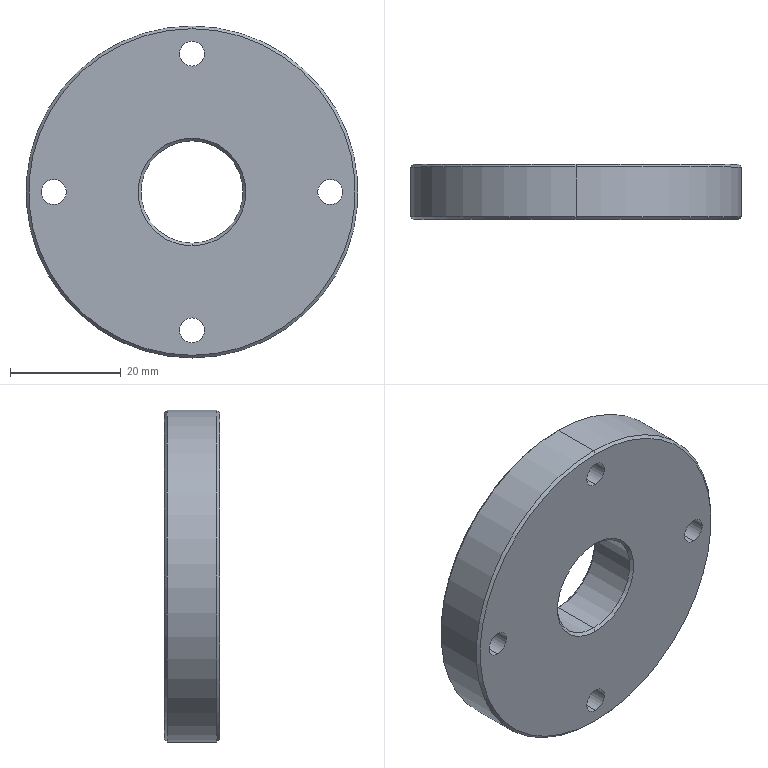Part | SolidWorks | features HoleWzd 2, Chamfer 1, Extrusion 1 | 1 solid | 34 faces | box 60 x 10 x 60 mm | volume 24256 mm3 | cylinder 20 | cone 8 | plane 6 | commonest cylinder face diameters 4.5 x8 8 x8 18.5 x2 60 x2
STEP:
#1=CARTESIAN_POINT('',(0.,10.,29.5));
#2=VERTEX_POINT('',#1);
#3=CARTESIAN_POINT('',(0.,10.,-29.5));
#4=VERTEX_POINT('',#3);
#5=CARTESIAN_POINT('',(0.,10.,0.));
#6=DIRECTION('',(0.,1.,0.));
#7=DIRECTION('',(0.,0.,1.));
#8=AXIS2_PLACEMENT_3D('',#5,#6,#7);
#9=CIRCLE('',#8,29.5);
#10=EDGE_CURVE('',#2,#4,#9,.T.);
#11=ORIENTED_EDGE('',*,*,#10,.F.);
#12=CARTESIAN_POINT('',(0.,9.5,30.));
#13=VERTEX_POINT('',#12);
#14=CARTESIAN_POINT('',(0.,10.,29.5));
#15=DIRECTION('',(0.,-0.7071,0.7071));
#16=VECTOR('',#15,1000.);
#17=LINE('',#14,#16);
#18=EDGE_CURVE('',#2,#13,#17,.T.);
#19=ORIENTED_EDGE('',*,*,#18,.T.);
#20=CARTESIAN_POINT('',(0.,9.5,-30.));
#21=VERTEX_POINT('',#20);
#22=CARTESIAN_POINT('',(0.,9.5,0.));
#23=DIRECTION('',(0.,-1.,0.));
#24=DIRECTION('',(0.,0.,1.));
#25=AXIS2_PLACEMENT_3D('',#22,#23,#24);
#26=CIRCLE('',#25,30.);
#27=EDGE_CURVE('',#21,#13,#26,.T.);
#28=ORIENTED_EDGE('',*,*,#27,.F.);
#29=CARTESIAN_POINT('',(0.,10.,-29.5));
#30=DIRECTION('',(0.,-0.7071,-0.7071));
#31=VECTOR('',#30,1000.);
#32=LINE('',#29,#31);
#33=EDGE_CURVE('',#4,#21,#32,.T.);
#34=ORIENTED_EDGE('',*,*,#33,.F.);
#35=EDGE_LOOP('',(#11,#19,#28,#34));
#36=FACE_OUTER_BOUND('',#35,.T.);
#37=CARTESIAN_POINT('',(0.,10.,0.));
#38=DIRECTION('',(0.,-1.,0.));
#39=DIRECTION('',(0.,0.,-1.));
#40=AXIS2_PLACEMENT_3D('',#37,#38,#39);
#41=CONICAL_SURFACE('',#40,29.5,0.7854);
#42=ADVANCED_FACE('',(#36),#41,.T.);
#43=CARTESIAN_POINT('',(0.,0.,-29.5));
#44=VERTEX_POINT('',#43);
#45=CARTESIAN_POINT('',(0.,0.,29.5));
#46=VERTEX_POINT('',#45);
#47=CARTESIAN_POINT('',(0.,0.,0.));
#48=DIRECTION('',(0.,-1.,0.));
#49=DIRECTION('',(0.,0.,1.));
#50=AXIS2_PLACEMENT_3D('',#47,#48,#49);
#51=CIRCLE('',#50,29.5);
#52=EDGE_CURVE('',#44,#46,#51,.T.);
#53=ORIENTED_EDGE('',*,*,#52,.F.);
#54=CARTESIAN_POINT('',(0.,0.5,-30.));
#55=VERTEX_POINT('',#54);
#56=CARTESIAN_POINT('',(0.,0.5,-30.));
#57=DIRECTION('',(0.,0.7071,-0.7071));
#58=VECTOR('',#57,1000.);
#59=LINE('',#56,#58);
#60=EDGE_CURVE('',#44,#55,#59,.T.);
#61=ORIENTED_EDGE('',*,*,#60,.T.);
#62=CARTESIAN_POINT('',(0.,0.5,30.));
#63=VERTEX_POINT('',#62);
#64=CARTESIAN_POINT('',(0.,0.5,0.));
#65=DIRECTION('',(0.,1.,0.));
#66=DIRECTION('',(0.,0.,1.));
#67=AXIS2_PLACEMENT_3D('',#64,#65,#66);
#68=CIRCLE('',#67,30.);
#69=EDGE_CURVE('',#63,#55,#68,.T.);
#70=ORIENTED_EDGE('',*,*,#69,.F.);
#71=CARTESIAN_POINT('',(0.,0.5,30.));
#72=DIRECTION('',(0.,0.7071,0.7071));
#73=VECTOR('',#72,1000.);
#74=LINE('',#71,#73);
#75=EDGE_CURVE('',#46,#63,#74,.T.);
#76=ORIENTED_EDGE('',*,*,#75,.F.);
#77=EDGE_LOOP('',(#53,#61,#70,#76));
#78=FACE_OUTER_BOUND('',#77,.T.);
#79=CARTESIAN_POINT('',(0.,0.5,0.));
#80=DIRECTION('',(0.,1.,0.));
#81=DIRECTION('',(0.,0.,1.));
#82=AXIS2_PLACEMENT_3D('',#79,#80,#81);
#83=CONICAL_SURFACE('',#82,30.,0.7854);
#84=ADVANCED_FACE('',(#78),#83,.T.);
#85=CARTESIAN_POINT('',(0.,9.5,-9.25));
#86=VERTEX_POINT('',#85);
#87=CARTESIAN_POINT('',(0.,9.5,9.25));
#88=VERTEX_POINT('',#87);
#89=CARTESIAN_POINT('',(0.,9.5,0.));
#90=DIRECTION('',(0.,1.,0.));
#91=DIRECTION('',(0.,0.,1.));
#92=AXIS2_PLACEMENT_3D('',#89,#90,#91);
#93=CIRCLE('',#92,9.25);
#94=EDGE_CURVE('',#86,#88,#93,.T.);
#95=ORIENTED_EDGE('',*,*,#94,.F.);
#96=CARTESIAN_POINT('',(0.,10.,-9.75));
#97=VERTEX_POINT('',#96);
#98=CARTESIAN_POINT('',(0.,9.5,-9.25));
#99=DIRECTION('',(0.,0.7071,-0.7071));
#100=VECTOR('',#99,1000.);
#101=LINE('',#98,#100);
#102=EDGE_CURVE('',#86,#97,#101,.T.);
#103=ORIENTED_EDGE('',*,*,#102,.T.);
#104=CARTESIAN_POINT('',(0.,10.,9.75));
#105=VERTEX_POINT('',#104);
#106=CARTESIAN_POINT('',(0.,10.,0.));
#107=DIRECTION('',(0.,-1.,0.));
#108=DIRECTION('',(0.,0.,1.));
#109=AXIS2_PLACEMENT_3D('',#106,#107,#108);
#110=CIRCLE('',#109,9.75);
#111=EDGE_CURVE('',#105,#97,#110,.T.);
#112=ORIENTED_EDGE('',*,*,#111,.F.);
#113=CARTESIAN_POINT('',(0.,9.5,9.25));
#114=DIRECTION('',(0.,0.7071,0.7071));
#115=VECTOR('',#114,1000.);
#116=LINE('',#113,#115);
#117=EDGE_CURVE('',#88,#105,#116,.T.);
#118=ORIENTED_EDGE('',*,*,#117,.F.);
#119=EDGE_LOOP('',(#95,#103,#112,#118));
#120=FACE_OUTER_BOUND('',#119,.T.);
#121=CARTESIAN_POINT('',(0.,9.5,0.));
#122=DIRECTION('',(0.,1.,0.));
#123=DIRECTION('',(0.,0.,1.));
#124=AXIS2_PLACEMENT_3D('',#121,#122,#123);
#125=CONICAL_SURFACE('',#124,9.25,0.7854);
#126=ADVANCED_FACE('',(#120),#125,.F.);
#127=CARTESIAN_POINT('',(0.,0.5,9.25));
#128=VERTEX_POINT('',#127);
#129=CARTESIAN_POINT('',(0.,0.5,-9.25));
#130=VERTEX_POINT('',#129);
#131=CARTESIAN_POINT('',(0.,0.5,0.));
#132=DIRECTION('',(0.,-1.,0.));
#133=DIRECTION('',(0.,0.,1.));
#134=AXIS2_PLACEMENT_3D('',#131,#132,#133);
#135=CIRCLE('',#134,9.25);
#136=EDGE_CURVE('',#128,#130,#135,.T.);
#137=ORIENTED_EDGE('',*,*,#136,.F.);
#138=CARTESIAN_POINT('',(0.,0.,9.75));
#139=VERTEX_POINT('',#138);
#140=CARTESIAN_POINT('',(0.,0.,9.75));
#141=DIRECTION('',(0.,-0.7071,0.7071));
#142=VECTOR('',#141,1000.);
#143=LINE('',#140,#142);
#144=EDGE_CURVE('',#128,#139,#143,.T.);
#145=ORIENTED_EDGE('',*,*,#144,.T.);
#146=CARTESIAN_POINT('',(0.,0.,-9.75));
#147=VERTEX_POINT('',#146);
#148=CARTESIAN_POINT('',(0.,0.,0.));
#149=DIRECTION('',(0.,1.,0.));
#150=DIRECTION('',(0.,0.,1.));
#151=AXIS2_PLACEMENT_3D('',#148,#149,#150);
#152=CIRCLE('',#151,9.75);
#153=EDGE_CURVE('',#147,#139,#152,.T.);
#154=ORIENTED_EDGE('',*,*,#153,.F.);
#155=CARTESIAN_POINT('',(0.,0.,-9.75));
#156=DIRECTION('',(0.,-0.7071,-0.7071));
#157=VECTOR('',#156,1000.);
#158=LINE('',#155,#157);
#159=EDGE_CURVE('',#130,#147,#158,.T.);
#160=ORIENTED_EDGE('',*,*,#159,.F.);
#161=EDGE_LOOP('',(#137,#145,#154,#160));
#162=FACE_OUTER_BOUND('',#161,.T.);
#163=CARTESIAN_POINT('',(0.,0.,0.));
#164=DIRECTION('',(0.,-1.,0.));
#165=DIRECTION('',(0.,0.,-1.));
#166=AXIS2_PLACEMENT_3D('',#163,#164,#165);
#167=CONICAL_SURFACE('',#166,9.75,0.7854);
#168=ADVANCED_FACE('',(#162),#167,.F.);
#169=CARTESIAN_POINT('',(0.,5.4,-29.));
#170=VERTEX_POINT('',#169);
#171=CARTESIAN_POINT('',(0.,5.4,-21.));
#172=VERTEX_POINT('',#171);
#173=CARTESIAN_POINT('',(0.,5.4,-25.));
#174=DIRECTION('',(0.,1.,0.));
#175=DIRECTION('',(0.,0.,1.));
#176=AXIS2_PLACEMENT_3D('',#173,#174,#175);
#177=CIRCLE('',#176,4.);
#178=EDGE_CURVE('',#170,#172,#177,.T.);
#179=ORIENTED_EDGE('',*,*,#178,.F.);
#180=CARTESIAN_POINT('',(0.,10.,-29.));
#181=VERTEX_POINT('',#180);
#182=CARTESIAN_POINT('',(0.,10.,-29.));
#183=DIRECTION('',(0.,1.,0.));
#184=VECTOR('',#183,1000.);
#185=LINE('',#182,#184);
#186=EDGE_CURVE('',#170,#181,#185,.T.);
#187=ORIENTED_EDGE('',*,*,#186,.T.);
#188=CARTESIAN_POINT('',(0.,10.,-21.));
#189=VERTEX_POINT('',#188);
#190=CARTESIAN_POINT('',(0.,10.,-25.));
#191=DIRECTION('',(0.,1.,0.));
#192=DIRECTION('',(0.,0.,1.));
#193=AXIS2_PLACEMENT_3D('',#190,#191,#192);
#194=CIRCLE('',#193,4.);
#195=EDGE_CURVE('',#181,#189,#194,.T.);
#196=ORIENTED_EDGE('',*,*,#195,.T.);
#197=CARTESIAN_POINT('',(0.,10.,-21.));
#198=DIRECTION('',(0.,1.,0.));
#199=VECTOR('',#198,1000.);
#200=LINE('',#197,#199);
#201=EDGE_CURVE('',#172,#189,#200,.T.);
#202=ORIENTED_EDGE('',*,*,#201,.F.);
#203=EDGE_LOOP('',(#179,#187,#196,#202));
#204=FACE_OUTER_BOUND('',#203,.T.);
#205=CARTESIAN_POINT('',(0.,10.,-25.));
#206=DIRECTION('',(0.,1.,0.));
#207=DIRECTION('',(0.,0.,1.));
#208=AXIS2_PLACEMENT_3D('',#205,#206,#207);
#209=CYLINDRICAL_SURFACE('',#208,4.);
#210=ADVANCED_FACE('',(#204),#209,.F.);
#211=CARTESIAN_POINT('',(0.,0.,-27.25));
#212=VERTEX_POINT('',#211);
#213=CARTESIAN_POINT('',(0.,0.,-22.75));
#214=VERTEX_POINT('',#213);
#215=CARTESIAN_POINT('',(0.,0.,-25.));
#216=DIRECTION('',(0.,1.,0.));
#217=DIRECTION('',(0.,0.,1.));
#218=AXIS2_PLACEMENT_3D('',#215,#216,#217);
#219=CIRCLE('',#218,2.25);
#220=EDGE_CURVE('',#212,#214,#219,.T.);
#221=ORIENTED_EDGE('',*,*,#220,.F.);
#222=CARTESIAN_POINT('',(0.,5.4,-27.25));
#223=VERTEX_POINT('',#222);
#224=CARTESIAN_POINT('',(0.,10.,-27.25));
#225=DIRECTION('',(0.,1.,0.));
#226=VECTOR('',#225,1000.);
#227=LINE('',#224,#226);
#228=EDGE_CURVE('',#212,#223,#227,.T.);
#229=ORIENTED_EDGE('',*,*,#228,.T.);
#230=CARTESIAN_POINT('',(0.,5.4,-22.75));
#231=VERTEX_POINT('',#230);
#232=CARTESIAN_POINT('',(0.,5.4,-25.));
#233=DIRECTION('',(0.,1.,0.));
#234=DIRECTION('',(0.,0.,1.));
#235=AXIS2_PLACEMENT_3D('',#232,#233,#234);
#236=CIRCLE('',#235,2.25);
#237=EDGE_CURVE('',#223,#231,#236,.T.);
#238=ORIENTED_EDGE('',*,*,#237,.T.);
#239=CARTESIAN_POINT('',(0.,10.,-22.75));
#240=DIRECTION('',(0.,1.,0.));
#241=VECTOR('',#240,1000.);
#242=LINE('',#239,#241);
#243=EDGE_CURVE('',#214,#231,#242,.T.);
#244=ORIENTED_EDGE('',*,*,#243,.F.);
#245=EDGE_LOOP('',(#221,#229,#238,#244));
#246=FACE_OUTER_BOUND('',#245,.T.);
#247=CARTESIAN_POINT('',(0.,10.,-25.));
#248=DIRECTION('',(0.,1.,0.));
#249=DIRECTION('',(0.,0.,1.));
#250=AXIS2_PLACEMENT_3D('',#247,#248,#249);
#251=CYLINDRICAL_SURFACE('',#250,2.25);
#252=ADVANCED_FACE('',(#246),#251,.F.);
#253=CARTESIAN_POINT('',(25.,5.4,-4.));
#254=VERTEX_POINT('',#253);
#255=CARTESIAN_POINT('',(25.,5.4,4.));
#256=VERTEX_POINT('',#255);
#257=CARTESIAN_POINT('',(25.,5.4,0.));
#258=DIRECTION('',(0.,1.,0.));
#259=DIRECTION('',(0.,0.,1.));
#260=AXIS2_PLACEMENT_3D('',#257,#258,#259);
#261=CIRCLE('',#260,4.);
#262=EDGE_CURVE('',#254,#256,#261,.T.);
#263=ORIENTED_EDGE('',*,*,#262,.F.);
#264=CARTESIAN_POINT('',(25.,10.,-4.));
#265=VERTEX_POINT('',#264);
#266=CARTESIAN_POINT('',(25.,10.,-4.));
#267=DIRECTION('',(0.,1.,0.));
#268=VECTOR('',#267,1000.);
#269=LINE('',#266,#268);
#270=EDGE_CURVE('',#254,#265,#269,.T.);
#271=ORIENTED_EDGE('',*,*,#270,.T.);
#272=CARTESIAN_POINT('',(25.,10.,4.));
#273=VERTEX_POINT('',#272);
#274=CARTESIAN_POINT('',(25.,10.,0.));
#275=DIRECTION('',(0.,1.,0.));
#276=DIRECTION('',(0.,0.,1.));
#277=AXIS2_PLACEMENT_3D('',#274,#275,#276);
#278=CIRCLE('',#277,4.);
#279=EDGE_CURVE('',#265,#273,#278,.T.);
#280=ORIENTED_EDGE('',*,*,#279,.T.);
#281=CARTESIAN_POINT('',(25.,10.,4.));
#282=DIRECTION('',(0.,1.,0.));
#283=VECTOR('',#282,1000.);
#284=LINE('',#281,#283);
#285=EDGE_CURVE('',#256,#273,#284,.T.);
#286=ORIENTED_EDGE('',*,*,#285,.F.);
#287=EDGE_LOOP('',(#263,#271,#280,#286));
#288=FACE_OUTER_BOUND('',#287,.T.);
#289=CARTESIAN_POINT('',(25.,10.,0.));
#290=DIRECTION('',(0.,1.,0.));
#291=DIRECTION('',(0.,0.,1.));
#292=AXIS2_PLACEMENT_3D('',#289,#290,#291);
#293=CYLINDRICAL_SURFACE('',#292,4.);
#294=ADVANCED_FACE('',(#288),#293,.F.);
#295=CARTESIAN_POINT('',(25.,0.,-2.25));
#296=VERTEX_POINT('',#295);
#297=CARTESIAN_POINT('',(25.,0.,2.25));
#298=VERTEX_POINT('',#297);
#299=CARTESIAN_POINT('',(25.,0.,0.));
#300=DIRECTION('',(0.,1.,0.));
#301=DIRECTION('',(0.,0.,1.));
#302=AXIS2_PLACEMENT_3D('',#299,#300,#301);
#303=CIRCLE('',#302,2.25);
#304=EDGE_CURVE('',#296,#298,#303,.T.);
#305=ORIENTED_EDGE('',*,*,#304,.F.);
#306=CARTESIAN_POINT('',(25.,5.4,-2.25));
#307=VERTEX_POINT('',#306);
#308=CARTESIAN_POINT('',(25.,10.,-2.25));
#309=DIRECTION('',(0.,1.,0.));
#310=VECTOR('',#309,1000.);
#311=LINE('',#308,#310);
#312=EDGE_CURVE('',#296,#307,#311,.T.);
#313=ORIENTED_EDGE('',*,*,#312,.T.);
#314=CARTESIAN_POINT('',(25.,5.4,2.25));
#315=VERTEX_POINT('',#314);
#316=CARTESIAN_POINT('',(25.,5.4,0.));
#317=DIRECTION('',(0.,1.,0.));
#318=DIRECTION('',(0.,0.,1.));
#319=AXIS2_PLACEMENT_3D('',#316,#317,#318);
#320=CIRCLE('',#319,2.25);
#321=EDGE_CURVE('',#307,#315,#320,.T.);
#322=ORIENTED_EDGE('',*,*,#321,.T.);
#323=CARTESIAN_POINT('',(25.,10.,2.25));
#324=DIRECTION('',(0.,1.,0.));
#325=VECTOR('',#324,1000.);
#326=LINE('',#323,#325);
#327=EDGE_CURVE('',#298,#315,#326,.T.);
#328=ORIENTED_EDGE('',*,*,#327,.F.);
#329=EDGE_LOOP('',(#305,#313,#322,#328));
#330=FACE_OUTER_BOUND('',#329,.T.);
#331=CARTESIAN_POINT('',(25.,10.,0.));
#332=DIRECTION('',(0.,1.,0.));
#333=DIRECTION('',(0.,0.,1.));
#334=AXIS2_PLACEMENT_3D('',#331,#332,#333);
#335=CYLINDRICAL_SURFACE('',#334,2.25);
#336=ADVANCED_FACE('',(#330),#335,.F.);
#337=CARTESIAN_POINT('',(0.,5.4,21.));
#338=VERTEX_POINT('',#337);
#339=CARTESIAN_POINT('',(0.,5.4,29.));
#340=VERTEX_POINT('',#339);
#341=CARTESIAN_POINT('',(0.,5.4,25.));
#342=DIRECTION('',(0.,1.,0.));
#343=DIRECTION('',(0.,0.,1.));
#344=AXIS2_PLACEMENT_3D('',#341,#342,#343);
#345=CIRCLE('',#344,4.);
#346=EDGE_CURVE('',#338,#340,#345,.T.);
#347=ORIENTED_EDGE('',*,*,#346,.F.);
#348=CARTESIAN_POINT('',(0.,10.,21.));
#349=VERTEX_POINT('',#348);
#350=CARTESIAN_POINT('',(0.,10.,21.));
#351=DIRECTION('',(0.,1.,0.));
#352=VECTOR('',#351,1000.);
#353=LINE('',#350,#352);
#354=EDGE_CURVE('',#338,#349,#353,.T.);
#355=ORIENTED_EDGE('',*,*,#354,.T.);
#356=CARTESIAN_POINT('',(0.,10.,29.));
#357=VERTEX_POINT('',#356);
#358=CARTESIAN_POINT('',(0.,10.,25.));
#359=DIRECTION('',(0.,1.,0.));
#360=DIRECTION('',(0.,0.,1.));
#361=AXIS2_PLACEMENT_3D('',#358,#359,#360);
#362=CIRCLE('',#361,4.);
#363=EDGE_CURVE('',#349,#357,#362,.T.);
#364=ORIENTED_EDGE('',*,*,#363,.T.);
#365=CARTESIAN_POINT('',(0.,10.,29.));
#366=DIRECTION('',(0.,1.,0.));
#367=VECTOR('',#366,1000.);
#368=LINE('',#365,#367);
#369=EDGE_CURVE('',#340,#357,#368,.T.);
#370=ORIENTED_EDGE('',*,*,#369,.F.);
#371=EDGE_LOOP('',(#347,#355,#364,#370));
#372=FACE_OUTER_BOUND('',#371,.T.);
#373=CARTESIAN_POINT('',(0.,10.,25.));
#374=DIRECTION('',(0.,1.,0.));
#375=DIRECTION('',(0.,0.,1.));
#376=AXIS2_PLACEMENT_3D('',#373,#374,#375);
#377=CYLINDRICAL_SURFACE('',#376,4.);
#378=ADVANCED_FACE('',(#372),#377,.F.);
#379=CARTESIAN_POINT('',(0.,0.,22.75));
#380=VERTEX_POINT('',#379);
#381=CARTESIAN_POINT('',(0.,0.,27.25));
#382=VERTEX_POINT('',#381);
#383=CARTESIAN_POINT('',(0.,0.,25.));
#384=DIRECTION('',(0.,1.,0.));
#385=DIRECTION('',(0.,0.,1.));
#386=AXIS2_PLACEMENT_3D('',#383,#384,#385);
#387=CIRCLE('',#386,2.25);
#388=EDGE_CURVE('',#380,#382,#387,.T.);
#389=ORIENTED_EDGE('',*,*,#388,.F.);
#390=CARTESIAN_POINT('',(0.,5.4,22.75));
#391=VERTEX_POINT('',#390);
#392=CARTESIAN_POINT('',(0.,10.,22.75));
#393=DIRECTION('',(0.,1.,0.));
#394=VECTOR('',#393,1000.);
#395=LINE('',#392,#394);
#396=EDGE_CURVE('',#380,#391,#395,.T.);
#397=ORIENTED_EDGE('',*,*,#396,.T.);
#398=CARTESIAN_POINT('',(0.,5.4,27.25));
#399=VERTEX_POINT('',#398);
#400=CARTESIAN_POINT('',(0.,5.4,25.));
#401=DIRECTION('',(0.,1.,0.));
#402=DIRECTION('',(0.,0.,1.));
#403=AXIS2_PLACEMENT_3D('',#400,#401,#402);
#404=CIRCLE('',#403,2.25);
#405=EDGE_CURVE('',#391,#399,#404,.T.);
#406=ORIENTED_EDGE('',*,*,#405,.T.);
#407=CARTESIAN_POINT('',(0.,10.,27.25));
#408=DIRECTION('',(0.,1.,0.));
#409=VECTOR('',#408,1000.);
#410=LINE('',#407,#409);
#411=EDGE_CURVE('',#382,#399,#410,.T.);
#412=ORIENTED_EDGE('',*,*,#411,.F.);
#413=EDGE_LOOP('',(#389,#397,#406,#412));
#414=FACE_OUTER_BOUND('',#413,.T.);
#415=CARTESIAN_POINT('',(0.,10.,25.));
#416=DIRECTION('',(0.,1.,0.));
#417=DIRECTION('',(0.,0.,1.));
#418=AXIS2_PLACEMENT_3D('',#415,#416,#417);
#419=CYLINDRICAL_SURFACE('',#418,2.25);
#420=ADVANCED_FACE('',(#414),#419,.F.);
#421=CARTESIAN_POINT('',(-25.,5.4,-4.));
#422=VERTEX_POINT('',#421);
#423=CARTESIAN_POINT('',(-25.,5.4,4.));
#424=VERTEX_POINT('',#423);
#425=CARTESIAN_POINT('',(-25.,5.4,0.));
#426=DIRECTION('',(0.,1.,0.));
#427=DIRECTION('',(0.,0.,1.));
#428=AXIS2_PLACEMENT_3D('',#425,#426,#427);
#429=CIRCLE('',#428,4.);
#430=EDGE_CURVE('',#422,#424,#429,.T.);
#431=ORIENTED_EDGE('',*,*,#430,.F.);
#432=CARTESIAN_POINT('',(-25.,10.,-4.));
#433=VERTEX_POINT('',#432);
#434=CARTESIAN_POINT('',(-25.,10.,-4.));
#435=DIRECTION('',(0.,1.,0.));
#436=VECTOR('',#435,1000.);
#437=LINE('',#434,#436);
#438=EDGE_CURVE('',#422,#433,#437,.T.);
#439=ORIENTED_EDGE('',*,*,#438,.T.);
#440=CARTESIAN_POINT('',(-25.,10.,4.));
#441=VERTEX_POINT('',#440);
#442=CARTESIAN_POINT('',(-25.,10.,0.));
#443=DIRECTION('',(0.,1.,0.));
#444=DIRECTION('',(0.,0.,1.));
#445=AXIS2_PLACEMENT_3D('',#442,#443,#444);
#446=CIRCLE('',#445,4.);
#447=EDGE_CURVE('',#433,#441,#446,.T.);
#448=ORIENTED_EDGE('',*,*,#447,.T.);
#449=CARTESIAN_POINT('',(-25.,10.,4.));
#450=DIRECTION('',(0.,1.,0.));
#451=VECTOR('',#450,1000.);
#452=LINE('',#449,#451);
#453=EDGE_CURVE('',#424,#441,#452,.T.);
#454=ORIENTED_EDGE('',*,*,#453,.F.);
#455=EDGE_LOOP('',(#431,#439,#448,#454));
#456=FACE_OUTER_BOUND('',#455,.T.);
#457=CARTESIAN_POINT('',(-25.,10.,0.));
#458=DIRECTION('',(0.,1.,0.));
#459=DIRECTION('',(0.,0.,1.));
#460=AXIS2_PLACEMENT_3D('',#457,#458,#459);
#461=CYLINDRICAL_SURFACE('',#460,4.);
#462=ADVANCED_FACE('',(#456),#461,.F.);
#463=CARTESIAN_POINT('',(-25.,0.,-2.25));
#464=VERTEX_POINT('',#463);
#465=CARTESIAN_POINT('',(-25.,0.,2.25));
#466=VERTEX_POINT('',#465);
#467=CARTESIAN_POINT('',(-25.,0.,0.));
#468=DIRECTION('',(0.,1.,0.));
#469=DIRECTION('',(0.,0.,1.));
#470=AXIS2_PLACEMENT_3D('',#467,#468,#469);
#471=CIRCLE('',#470,2.25);
#472=EDGE_CURVE('',#464,#466,#471,.T.);
#473=ORIENTED_EDGE('',*,*,#472,.F.);
#474=CARTESIAN_POINT('',(-25.,5.4,-2.25));
#475=VERTEX_POINT('',#474);
#476=CARTESIAN_POINT('',(-25.,10.,-2.25));
#477=DIRECTION('',(0.,1.,0.));
#478=VECTOR('',#477,1000.);
#479=LINE('',#476,#478);
#480=EDGE_CURVE('',#464,#475,#479,.T.);
#481=ORIENTED_EDGE('',*,*,#480,.T.);
#482=CARTESIAN_POINT('',(-25.,5.4,2.25));
#483=VERTEX_POINT('',#482);
#484=CARTESIAN_POINT('',(-25.,5.4,0.));
#485=DIRECTION('',(0.,1.,0.));
#486=DIRECTION('',(0.,0.,1.));
#487=AXIS2_PLACEMENT_3D('',#484,#485,#486);
#488=CIRCLE('',#487,2.25);
#489=EDGE_CURVE('',#475,#483,#488,.T.);
#490=ORIENTED_EDGE('',*,*,#489,.T.);
#491=CARTESIAN_POINT('',(-25.,10.,2.25));
#492=DIRECTION('',(0.,1.,0.));
#493=VECTOR('',#492,1000.);
#494=LINE('',#491,#493);
#495=EDGE_CURVE('',#466,#483,#494,.T.);
#496=ORIENTED_EDGE('',*,*,#495,.F.);
#497=EDGE_LOOP('',(#473,#481,#490,#496));
#498=FACE_OUTER_BOUND('',#497,.T.);
#499=CARTESIAN_POINT('',(-25.,10.,0.));
#500=DIRECTION('',(0.,1.,0.));
#501=DIRECTION('',(0.,0.,1.));
#502=AXIS2_PLACEMENT_3D('',#499,#500,#501);
#503=CYLINDRICAL_SURFACE('',#502,2.25);
#504=ADVANCED_FACE('',(#498),#503,.F.);
#505=ORIENTED_EDGE('',*,*,#136,.T.);
#506=CARTESIAN_POINT('',(0.,10.,-9.25));
#507=DIRECTION('',(0.,1.,0.));
#508=VECTOR('',#507,1000.);
#509=LINE('',#506,#508);
#510=EDGE_CURVE('',#130,#86,#509,.T.);
#511=ORIENTED_EDGE('',*,*,#510,.T.);
#512=ORIENTED_EDGE('',*,*,#94,.T.);
#513=CARTESIAN_POINT('',(0.,10.,9.25));
#514=DIRECTION('',(0.,1.,0.));
#515=VECTOR('',#514,1000.);
#516=LINE('',#513,#515);
#517=EDGE_CURVE('',#128,#88,#516,.T.);
#518=ORIENTED_EDGE('',*,*,#517,.F.);
#519=EDGE_LOOP('',(#505,#511,#512,#518));
#520=FACE_OUTER_BOUND('',#519,.T.);
#521=CARTESIAN_POINT('',(0.,10.,0.));
#522=DIRECTION('',(0.,1.,0.));
#523=DIRECTION('',(0.,0.,1.));
#524=AXIS2_PLACEMENT_3D('',#521,#522,#523);
#525=CYLINDRICAL_SURFACE('',#524,9.25);
#526=ADVANCED_FACE('',(#520),#525,.F.);
#527=ORIENTED_EDGE('',*,*,#27,.T.);
#528=CARTESIAN_POINT('',(0.,10.,30.));
#529=DIRECTION('',(0.,-1.,0.));
#530=VECTOR('',#529,1000.);
#531=LINE('',#528,#530);
#532=EDGE_CURVE('',#13,#63,#531,.T.);
#533=ORIENTED_EDGE('',*,*,#532,.T.);
#534=ORIENTED_EDGE('',*,*,#69,.T.);
#535=CARTESIAN_POINT('',(0.,10.,-30.));
#536=DIRECTION('',(0.,-1.,0.));
#537=VECTOR('',#536,1000.);
#538=LINE('',#535,#537);
#539=EDGE_CURVE('',#21,#55,#538,.T.);
#540=ORIENTED_EDGE('',*,*,#539,.F.);
#541=EDGE_LOOP('',(#527,#533,#534,#540));
#542=FACE_OUTER_BOUND('',#541,.T.);
#543=CARTESIAN_POINT('',(0.,10.,0.));
#544=DIRECTION('',(0.,-1.,0.));
#545=DIRECTION('',(0.,0.,-1.));
#546=AXIS2_PLACEMENT_3D('',#543,#544,#545);
#547=CYLINDRICAL_SURFACE('',#546,30.);
#548=ADVANCED_FACE('',(#542),#547,.T.);
#549=ORIENTED_EDGE('',*,*,#532,.F.);
#550=CARTESIAN_POINT('',(0.,9.5,0.));
#551=DIRECTION('',(0.,-1.,0.));
#552=DIRECTION('',(0.,0.,1.));
#553=AXIS2_PLACEMENT_3D('',#550,#551,#552);
#554=CIRCLE('',#553,30.);
#555=EDGE_CURVE('',#13,#21,#554,.T.);
#556=ORIENTED_EDGE('',*,*,#555,.T.);
#557=ORIENTED_EDGE('',*,*,#539,.T.);
#558=CARTESIAN_POINT('',(0.,0.5,0.));
#559=DIRECTION('',(0.,1.,0.));
#560=DIRECTION('',(0.,0.,1.));
#561=AXIS2_PLACEMENT_3D('',#558,#559,#560);
#562=CIRCLE('',#561,30.);
#563=EDGE_CURVE('',#55,#63,#562,.T.);
#564=ORIENTED_EDGE('',*,*,#563,.T.);
#565=EDGE_LOOP('',(#549,#556,#557,#564));
#566=FACE_OUTER_BOUND('',#565,.T.);
#567=CARTESIAN_POINT('',(0.,10.,0.));
#568=DIRECTION('',(0.,-1.,0.));
#569=DIRECTION('',(0.,0.,-1.));
#570=AXIS2_PLACEMENT_3D('',#567,#568,#569);
#571=CYLINDRICAL_SURFACE('',#570,30.);
#572=ADVANCED_FACE('',(#566),#571,.T.);
#573=ORIENTED_EDGE('',*,*,#111,.T.);
#574=CARTESIAN_POINT('',(0.,10.,0.));
#575=DIRECTION('',(0.,-1.,0.));
#576=DIRECTION('',(0.,0.,1.));
#577=AXIS2_PLACEMENT_3D('',#574,#575,#576);
#578=CIRCLE('',#577,9.75);
#579=EDGE_CURVE('',#97,#105,#578,.T.);
#580=ORIENTED_EDGE('',*,*,#579,.T.);
#581=EDGE_LOOP('',(#573,#580));
#582=FACE_BOUND('',#581,.T.);
#583=CARTESIAN_POINT('',(0.,10.,0.));
#584=DIRECTION('',(0.,1.,0.));
#585=DIRECTION('',(0.,0.,1.));
#586=AXIS2_PLACEMENT_3D('',#583,#584,#585);
#587=CIRCLE('',#586,29.5);
#588=EDGE_CURVE('',#4,#2,#587,.T.);
#589=ORIENTED_EDGE('',*,*,#588,.T.);
#590=ORIENTED_EDGE('',*,*,#10,.T.);
#591=EDGE_LOOP('',(#589,#590));
#592=FACE_OUTER_BOUND('',#591,.T.);
#593=CARTESIAN_POINT('',(0.,10.,-25.));
#594=DIRECTION('',(0.,1.,0.));
#595=DIRECTION('',(0.,0.,1.));
#596=AXIS2_PLACEMENT_3D('',#593,#594,#595);
#597=CIRCLE('',#596,4.);
#598=EDGE_CURVE('',#189,#181,#597,.T.);
#599=ORIENTED_EDGE('',*,*,#598,.F.);
#600=ORIENTED_EDGE('',*,*,#195,.F.);
#601=EDGE_LOOP('',(#599,#600));
#602=FACE_BOUND('',#601,.T.);
#603=CARTESIAN_POINT('',(25.,10.,0.));
#604=DIRECTION('',(0.,1.,0.));
#605=DIRECTION('',(0.,0.,1.));
#606=AXIS2_PLACEMENT_3D('',#603,#604,#605);
#607=CIRCLE('',#606,4.);
#608=EDGE_CURVE('',#273,#265,#607,.T.);
#609=ORIENTED_EDGE('',*,*,#608,.F.);
#610=ORIENTED_EDGE('',*,*,#279,.F.);
#611=EDGE_LOOP('',(#609,#610));
#612=FACE_BOUND('',#611,.T.);
#613=CARTESIAN_POINT('',(0.,10.,25.));
#614=DIRECTION('',(0.,1.,0.));
#615=DIRECTION('',(0.,0.,1.));
#616=AXIS2_PLACEMENT_3D('',#613,#614,#615);
#617=CIRCLE('',#616,4.);
#618=EDGE_CURVE('',#357,#349,#617,.T.);
#619=ORIENTED_EDGE('',*,*,#618,.F.);
#620=ORIENTED_EDGE('',*,*,#363,.F.);
#621=EDGE_LOOP('',(#619,#620));
#622=FACE_BOUND('',#621,.T.);
#623=CARTESIAN_POINT('',(-25.,10.,0.));
#624=DIRECTION('',(0.,1.,0.));
#625=DIRECTION('',(0.,0.,1.));
#626=AXIS2_PLACEMENT_3D('',#623,#624,#625);
#627=CIRCLE('',#626,4.);
#628=EDGE_CURVE('',#441,#433,#627,.T.);
#629=ORIENTED_EDGE('',*,*,#628,.F.);
#630=ORIENTED_EDGE('',*,*,#447,.F.);
#631=EDGE_LOOP('',(#629,#630));
#632=FACE_BOUND('',#631,.T.);
#633=CARTESIAN_POINT('',(0.,10.,0.));
#634=DIRECTION('',(0.,1.,0.));
#635=DIRECTION('',(0.,0.,1.));
#636=AXIS2_PLACEMENT_3D('',#633,#634,#635);
#637=PLANE('',#636);
#638=ADVANCED_FACE('',(#582,#592,#602,#612,#622,#632),#637,.T.);
#639=ORIENTED_EDGE('',*,*,#153,.T.);
#640=CARTESIAN_POINT('',(0.,0.,0.));
#641=DIRECTION('',(0.,1.,0.));
#642=DIRECTION('',(0.,0.,1.));
#643=AXIS2_PLACEMENT_3D('',#640,#641,#642);
#644=CIRCLE('',#643,9.75);
#645=EDGE_CURVE('',#139,#147,#644,.T.);
#646=ORIENTED_EDGE('',*,*,#645,.T.);
#647=EDGE_LOOP('',(#639,#646));
#648=FACE_BOUND('',#647,.T.);
#649=CARTESIAN_POINT('',(0.,0.,0.));
#650=DIRECTION('',(0.,-1.,0.));
#651=DIRECTION('',(0.,0.,1.));
#652=AXIS2_PLACEMENT_3D('',#649,#650,#651);
#653=CIRCLE('',#652,29.5);
#654=EDGE_CURVE('',#46,#44,#653,.T.);
#655=ORIENTED_EDGE('',*,*,#654,.T.);
#656=ORIENTED_EDGE('',*,*,#52,.T.);
#657=EDGE_LOOP('',(#655,#656));
#658=FACE_OUTER_BOUND('',#657,.T.);
#659=CARTESIAN_POINT('',(0.,0.,-25.));
#660=DIRECTION('',(0.,1.,0.));
#661=DIRECTION('',(0.,0.,1.));
#662=AXIS2_PLACEMENT_3D('',#659,#660,#661);
#663=CIRCLE('',#662,2.25);
#664=EDGE_CURVE('',#214,#212,#663,.T.);
#665=ORIENTED_EDGE('',*,*,#664,.T.);
#666=ORIENTED_EDGE('',*,*,#220,.T.);
#667=EDGE_LOOP('',(#665,#666));
#668=FACE_BOUND('',#667,.T.);
#669=CARTESIAN_POINT('',(25.,0.,0.));
#670=DIRECTION('',(0.,1.,0.));
#671=DIRECTION('',(0.,0.,1.));
#672=AXIS2_PLACEMENT_3D('',#669,#670,#671);
#673=CIRCLE('',#672,2.25);
#674=EDGE_CURVE('',#298,#296,#673,.T.);
#675=ORIENTED_EDGE('',*,*,#674,.T.);
#676=ORIENTED_EDGE('',*,*,#304,.T.);
#677=EDGE_LOOP('',(#675,#676));
#678=FACE_BOUND('',#677,.T.);
#679=CARTESIAN_POINT('',(0.,0.,25.));
#680=DIRECTION('',(0.,1.,0.));
#681=DIRECTION('',(0.,0.,1.));
#682=AXIS2_PLACEMENT_3D('',#679,#680,#681);
#683=CIRCLE('',#682,2.25);
#684=EDGE_CURVE('',#382,#380,#683,.T.);
#685=ORIENTED_EDGE('',*,*,#684,.T.);
#686=ORIENTED_EDGE('',*,*,#388,.T.);
#687=EDGE_LOOP('',(#685,#686));
#688=FACE_BOUND('',#687,.T.);
#689=CARTESIAN_POINT('',(-25.,0.,0.));
#690=DIRECTION('',(0.,1.,0.));
#691=DIRECTION('',(0.,0.,1.));
#692=AXIS2_PLACEMENT_3D('',#689,#690,#691);
#693=CIRCLE('',#692,2.25);
#694=EDGE_CURVE('',#466,#464,#693,.T.);
#695=ORIENTED_EDGE('',*,*,#694,.T.);
#696=ORIENTED_EDGE('',*,*,#472,.T.);
#697=EDGE_LOOP('',(#695,#696));
#698=FACE_BOUND('',#697,.T.);
#699=CARTESIAN_POINT('',(0.,0.,0.));
#700=DIRECTION('',(0.,1.,0.));
#701=DIRECTION('',(0.,0.,1.));
#702=AXIS2_PLACEMENT_3D('',#699,#700,#701);
#703=PLANE('',#702);
#704=ADVANCED_FACE('',(#648,#658,#668,#678,#688,#698),#703,.F.);
#705=ORIENTED_EDGE('',*,*,#510,.F.);
#706=CARTESIAN_POINT('',(0.,0.5,0.));
#707=DIRECTION('',(0.,-1.,0.));
#708=DIRECTION('',(0.,0.,1.));
#709=AXIS2_PLACEMENT_3D('',#706,#707,#708);
#710=CIRCLE('',#709,9.25);
#711=EDGE_CURVE('',#130,#128,#710,.T.);
#712=ORIENTED_EDGE('',*,*,#711,.T.);
#713=ORIENTED_EDGE('',*,*,#517,.T.);
#714=CARTESIAN_POINT('',(0.,9.5,0.));
#715=DIRECTION('',(0.,1.,0.));
#716=DIRECTION('',(0.,0.,1.));
#717=AXIS2_PLACEMENT_3D('',#714,#715,#716);
#718=CIRCLE('',#717,9.25);
#719=EDGE_CURVE('',#88,#86,#718,.T.);
#720=ORIENTED_EDGE('',*,*,#719,.T.);
#721=EDGE_LOOP('',(#705,#712,#713,#720));
#722=FACE_OUTER_BOUND('',#721,.T.);
#723=CARTESIAN_POINT('',(0.,10.,0.));
#724=DIRECTION('',(0.,1.,0.));
#725=DIRECTION('',(0.,0.,1.));
#726=AXIS2_PLACEMENT_3D('',#723,#724,#725);
#727=CYLINDRICAL_SURFACE('',#726,9.25);
#728=ADVANCED_FACE('',(#722),#727,.F.);
#729=ORIENTED_EDGE('',*,*,#480,.F.);
#730=ORIENTED_EDGE('',*,*,#694,.F.);
#731=ORIENTED_EDGE('',*,*,#495,.T.);
#732=CARTESIAN_POINT('',(-25.,5.4,0.));
#733=DIRECTION('',(0.,1.,0.));
#734=DIRECTION('',(0.,0.,1.));
#735=AXIS2_PLACEMENT_3D('',#732,#733,#734);
#736=CIRCLE('',#735,2.25);
#737=EDGE_CURVE('',#483,#475,#736,.T.);
#738=ORIENTED_EDGE('',*,*,#737,.T.);
#739=EDGE_LOOP('',(#729,#730,#731,#738));
#740=FACE_OUTER_BOUND('',#739,.T.);
#741=CARTESIAN_POINT('',(-25.,10.,0.));
#742=DIRECTION('',(0.,1.,0.));
#743=DIRECTION('',(0.,0.,1.));
#744=AXIS2_PLACEMENT_3D('',#741,#742,#743);
#745=CYLINDRICAL_SURFACE('',#744,2.25);
#746=ADVANCED_FACE('',(#740),#745,.F.);
#747=ORIENTED_EDGE('',*,*,#737,.F.);
#748=ORIENTED_EDGE('',*,*,#489,.F.);
#749=EDGE_LOOP('',(#747,#748));
#750=FACE_BOUND('',#749,.T.);
#751=CARTESIAN_POINT('',(-25.,5.4,0.));
#752=DIRECTION('',(0.,1.,0.));
#753=DIRECTION('',(0.,0.,1.));
#754=AXIS2_PLACEMENT_3D('',#751,#752,#753);
#755=CIRCLE('',#754,4.);
#756=EDGE_CURVE('',#424,#422,#755,.T.);
#757=ORIENTED_EDGE('',*,*,#756,.T.);
#758=ORIENTED_EDGE('',*,*,#430,.T.);
#759=EDGE_LOOP('',(#757,#758));
#760=FACE_OUTER_BOUND('',#759,.T.);
#761=CARTESIAN_POINT('',(-22.75,5.4,0.));
#762=DIRECTION('',(0.,-1.,0.));
#763=DIRECTION('',(0.,0.,-1.));
#764=AXIS2_PLACEMENT_3D('',#761,#762,#763);
#765=PLANE('',#764);
#766=ADVANCED_FACE('',(#750,#760),#765,.F.);
#767=ORIENTED_EDGE('',*,*,#438,.F.);
#768=ORIENTED_EDGE('',*,*,#756,.F.);
#769=ORIENTED_EDGE('',*,*,#453,.T.);
#770=ORIENTED_EDGE('',*,*,#628,.T.);
#771=EDGE_LOOP('',(#767,#768,#769,#770));
#772=FACE_OUTER_BOUND('',#771,.T.);
#773=CARTESIAN_POINT('',(-25.,10.,0.));
#774=DIRECTION('',(0.,1.,0.));
#775=DIRECTION('',(0.,0.,1.));
#776=AXIS2_PLACEMENT_3D('',#773,#774,#775);
#777=CYLINDRICAL_SURFACE('',#776,4.);
#778=ADVANCED_FACE('',(#772),#777,.F.);
#779=ORIENTED_EDGE('',*,*,#396,.F.);
#780=ORIENTED_EDGE('',*,*,#684,.F.);
#781=ORIENTED_EDGE('',*,*,#411,.T.);
#782=CARTESIAN_POINT('',(0.,5.4,25.));
#783=DIRECTION('',(0.,1.,0.));
#784=DIRECTION('',(0.,0.,1.));
#785=AXIS2_PLACEMENT_3D('',#782,#783,#784);
#786=CIRCLE('',#785,2.25);
#787=EDGE_CURVE('',#399,#391,#786,.T.);
#788=ORIENTED_EDGE('',*,*,#787,.T.);
#789=EDGE_LOOP('',(#779,#780,#781,#788));
#790=FACE_OUTER_BOUND('',#789,.T.);
#791=CARTESIAN_POINT('',(0.,10.,25.));
#792=DIRECTION('',(0.,1.,0.));
#793=DIRECTION('',(0.,0.,1.));
#794=AXIS2_PLACEMENT_3D('',#791,#792,#793);
#795=CYLINDRICAL_SURFACE('',#794,2.25);
#796=ADVANCED_FACE('',(#790),#795,.F.);
#797=ORIENTED_EDGE('',*,*,#787,.F.);
#798=ORIENTED_EDGE('',*,*,#405,.F.);
#799=EDGE_LOOP('',(#797,#798));
#800=FACE_BOUND('',#799,.T.);
#801=CARTESIAN_POINT('',(0.,5.4,25.));
#802=DIRECTION('',(0.,1.,0.));
#803=DIRECTION('',(0.,0.,1.));
#804=AXIS2_PLACEMENT_3D('',#801,#802,#803);
#805=CIRCLE('',#804,4.);
#806=EDGE_CURVE('',#340,#338,#805,.T.);
#807=ORIENTED_EDGE('',*,*,#806,.T.);
#808=ORIENTED_EDGE('',*,*,#346,.T.);
#809=EDGE_LOOP('',(#807,#808));
#810=FACE_OUTER_BOUND('',#809,.T.);
#811=CARTESIAN_POINT('',(2.25,5.4,25.));
#812=DIRECTION('',(0.,-1.,0.));
#813=DIRECTION('',(0.,0.,-1.));
#814=AXIS2_PLACEMENT_3D('',#811,#812,#813);
#815=PLANE('',#814);
#816=ADVANCED_FACE('',(#800,#810),#815,.F.);
#817=ORIENTED_EDGE('',*,*,#354,.F.);
#818=ORIENTED_EDGE('',*,*,#806,.F.);
#819=ORIENTED_EDGE('',*,*,#369,.T.);
#820=ORIENTED_EDGE('',*,*,#618,.T.);
#821=EDGE_LOOP('',(#817,#818,#819,#820));
#822=FACE_OUTER_BOUND('',#821,.T.);
#823=CARTESIAN_POINT('',(0.,10.,25.));
#824=DIRECTION('',(0.,1.,0.));
#825=DIRECTION('',(0.,0.,1.));
#826=AXIS2_PLACEMENT_3D('',#823,#824,#825);
#827=CYLINDRICAL_SURFACE('',#826,4.);
#828=ADVANCED_FACE('',(#822),#827,.F.);
#829=ORIENTED_EDGE('',*,*,#312,.F.);
#830=ORIENTED_EDGE('',*,*,#674,.F.);
#831=ORIENTED_EDGE('',*,*,#327,.T.);
#832=CARTESIAN_POINT('',(25.,5.4,0.));
#833=DIRECTION('',(0.,1.,0.));
#834=DIRECTION('',(0.,0.,1.));
#835=AXIS2_PLACEMENT_3D('',#832,#833,#834);
#836=CIRCLE('',#835,2.25);
#837=EDGE_CURVE('',#315,#307,#836,.T.);
#838=ORIENTED_EDGE('',*,*,#837,.T.);
#839=EDGE_LOOP('',(#829,#830,#831,#838));
#840=FACE_OUTER_BOUND('',#839,.T.);
#841=CARTESIAN_POINT('',(25.,10.,0.));
#842=DIRECTION('',(0.,1.,0.));
#843=DIRECTION('',(0.,0.,1.));
#844=AXIS2_PLACEMENT_3D('',#841,#842,#843);
#845=CYLINDRICAL_SURFACE('',#844,2.25);
#846=ADVANCED_FACE('',(#840),#845,.F.);
#847=ORIENTED_EDGE('',*,*,#837,.F.);
#848=ORIENTED_EDGE('',*,*,#321,.F.);
#849=EDGE_LOOP('',(#847,#848));
#850=FACE_BOUND('',#849,.T.);
#851=CARTESIAN_POINT('',(25.,5.4,0.));
#852=DIRECTION('',(0.,1.,0.));
#853=DIRECTION('',(0.,0.,1.));
#854=AXIS2_PLACEMENT_3D('',#851,#852,#853);
#855=CIRCLE('',#854,4.);
#856=EDGE_CURVE('',#256,#254,#855,.T.);
#857=ORIENTED_EDGE('',*,*,#856,.T.);
#858=ORIENTED_EDGE('',*,*,#262,.T.);
#859=EDGE_LOOP('',(#857,#858));
#860=FACE_OUTER_BOUND('',#859,.T.);
#861=CARTESIAN_POINT('',(27.25,5.4,0.));
#862=DIRECTION('',(0.,-1.,0.));
#863=DIRECTION('',(0.,0.,-1.));
#864=AXIS2_PLACEMENT_3D('',#861,#862,#863);
#865=PLANE('',#864);
#866=ADVANCED_FACE('',(#850,#860),#865,.F.);
#867=ORIENTED_EDGE('',*,*,#270,.F.);
#868=ORIENTED_EDGE('',*,*,#856,.F.);
#869=ORIENTED_EDGE('',*,*,#285,.T.);
#870=ORIENTED_EDGE('',*,*,#608,.T.);
#871=EDGE_LOOP('',(#867,#868,#869,#870));
#872=FACE_OUTER_BOUND('',#871,.T.);
#873=CARTESIAN_POINT('',(25.,10.,0.));
#874=DIRECTION('',(0.,1.,0.));
#875=DIRECTION('',(0.,0.,1.));
#876=AXIS2_PLACEMENT_3D('',#873,#874,#875);
#877=CYLINDRICAL_SURFACE('',#876,4.);
#878=ADVANCED_FACE('',(#872),#877,.F.);
#879=ORIENTED_EDGE('',*,*,#228,.F.);
#880=ORIENTED_EDGE('',*,*,#664,.F.);
#881=ORIENTED_EDGE('',*,*,#243,.T.);
#882=CARTESIAN_POINT('',(0.,5.4,-25.));
#883=DIRECTION('',(0.,1.,0.));
#884=DIRECTION('',(0.,0.,1.));
#885=AXIS2_PLACEMENT_3D('',#882,#883,#884);
#886=CIRCLE('',#885,2.25);
#887=EDGE_CURVE('',#231,#223,#886,.T.);
#888=ORIENTED_EDGE('',*,*,#887,.T.);
#889=EDGE_LOOP('',(#879,#880,#881,#888));
#890=FACE_OUTER_BOUND('',#889,.T.);
#891=CARTESIAN_POINT('',(0.,10.,-25.));
#892=DIRECTION('',(0.,1.,0.));
#893=DIRECTION('',(0.,0.,1.));
#894=AXIS2_PLACEMENT_3D('',#891,#892,#893);
#895=CYLINDRICAL_SURFACE('',#894,2.25);
#896=ADVANCED_FACE('',(#890),#895,.F.);
#897=ORIENTED_EDGE('',*,*,#887,.F.);
#898=ORIENTED_EDGE('',*,*,#237,.F.);
#899=EDGE_LOOP('',(#897,#898));
#900=FACE_BOUND('',#899,.T.);
#901=CARTESIAN_POINT('',(0.,5.4,-25.));
#902=DIRECTION('',(0.,1.,0.));
#903=DIRECTION('',(0.,0.,1.));
#904=AXIS2_PLACEMENT_3D('',#901,#902,#903);
#905=CIRCLE('',#904,4.);
#906=EDGE_CURVE('',#172,#170,#905,.T.);
#907=ORIENTED_EDGE('',*,*,#906,.T.);
#908=ORIENTED_EDGE('',*,*,#178,.T.);
#909=EDGE_LOOP('',(#907,#908));
#910=FACE_OUTER_BOUND('',#909,.T.);
#911=CARTESIAN_POINT('',(2.25,5.4,-25.));
#912=DIRECTION('',(0.,-1.,0.));
#913=DIRECTION('',(0.,0.,-1.));
#914=AXIS2_PLACEMENT_3D('',#911,#912,#913);
#915=PLANE('',#914);
#916=ADVANCED_FACE('',(#900,#910),#915,.F.);
#917=ORIENTED_EDGE('',*,*,#186,.F.);
#918=ORIENTED_EDGE('',*,*,#906,.F.);
#919=ORIENTED_EDGE('',*,*,#201,.T.);
#920=ORIENTED_EDGE('',*,*,#598,.T.);
#921=EDGE_LOOP('',(#917,#918,#919,#920));
#922=FACE_OUTER_BOUND('',#921,.T.);
#923=CARTESIAN_POINT('',(0.,10.,-25.));
#924=DIRECTION('',(0.,1.,0.));
#925=DIRECTION('',(0.,0.,1.));
#926=AXIS2_PLACEMENT_3D('',#923,#924,#925);
#927=CYLINDRICAL_SURFACE('',#926,4.);
#928=ADVANCED_FACE('',(#922),#927,.F.);
#929=ORIENTED_EDGE('',*,*,#144,.F.);
#930=ORIENTED_EDGE('',*,*,#711,.F.);
#931=ORIENTED_EDGE('',*,*,#159,.T.);
#932=ORIENTED_EDGE('',*,*,#645,.F.);
#933=EDGE_LOOP('',(#929,#930,#931,#932));
#934=FACE_OUTER_BOUND('',#933,.T.);
#935=CARTESIAN_POINT('',(0.,0.,0.));
#936=DIRECTION('',(0.,-1.,0.));
#937=DIRECTION('',(0.,0.,-1.));
#938=AXIS2_PLACEMENT_3D('',#935,#936,#937);
#939=CONICAL_SURFACE('',#938,9.75,0.7854);
#940=ADVANCED_FACE('',(#934),#939,.F.);
#941=ORIENTED_EDGE('',*,*,#102,.F.);
#942=ORIENTED_EDGE('',*,*,#719,.F.);
#943=ORIENTED_EDGE('',*,*,#117,.T.);
#944=ORIENTED_EDGE('',*,*,#579,.F.);
#945=EDGE_LOOP('',(#941,#942,#943,#944));
#946=FACE_OUTER_BOUND('',#945,.T.);
#947=CARTESIAN_POINT('',(0.,9.5,0.));
#948=DIRECTION('',(0.,1.,0.));
#949=DIRECTION('',(0.,0.,1.));
#950=AXIS2_PLACEMENT_3D('',#947,#948,#949);
#951=CONICAL_SURFACE('',#950,9.25,0.7854);
#952=ADVANCED_FACE('',(#946),#951,.F.);
#953=ORIENTED_EDGE('',*,*,#60,.F.);
#954=ORIENTED_EDGE('',*,*,#654,.F.);
#955=ORIENTED_EDGE('',*,*,#75,.T.);
#956=ORIENTED_EDGE('',*,*,#563,.F.);
#957=EDGE_LOOP('',(#953,#954,#955,#956));
#958=FACE_OUTER_BOUND('',#957,.T.);
#959=CARTESIAN_POINT('',(0.,0.5,0.));
#960=DIRECTION('',(0.,1.,0.));
#961=DIRECTION('',(0.,0.,1.));
#962=AXIS2_PLACEMENT_3D('',#959,#960,#961);
#963=CONICAL_SURFACE('',#962,30.,0.7854);
#964=ADVANCED_FACE('',(#958),#963,.T.);
#965=ORIENTED_EDGE('',*,*,#18,.F.);
#966=ORIENTED_EDGE('',*,*,#588,.F.);
#967=ORIENTED_EDGE('',*,*,#33,.T.);
#968=ORIENTED_EDGE('',*,*,#555,.F.);
#969=EDGE_LOOP('',(#965,#966,#967,#968));
#970=FACE_OUTER_BOUND('',#969,.T.);
#971=CARTESIAN_POINT('',(0.,10.,0.));
#972=DIRECTION('',(0.,-1.,0.));
#973=DIRECTION('',(0.,0.,-1.));
#974=AXIS2_PLACEMENT_3D('',#971,#972,#973);
#975=CONICAL_SURFACE('',#974,29.5,0.7854);
#976=ADVANCED_FACE('',(#970),#975,.T.);
#977=CLOSED_SHELL('',(#42,#84,#126,#168,#210,#252,#294,#336,#378,#420,#462,#504,#526,#548,#572,#638,#704,#728,#746,#766,#778,#796,#816,#828,#846,#866,#878,#896,#916,#928,#940,#952,#964,#976));
#978=MANIFOLD_SOLID_BREP('',#977);
#979=CARTESIAN_POINT('',(0.,0.,0.));
#980=DIRECTION('',(0.,0.,1.));
#981=DIRECTION('',(1.,0.,0.));
#982=AXIS2_PLACEMENT_3D('',#979,#980,#981);
#983=(LENGTH_UNIT()NAMED_UNIT(*)SI_UNIT(.MILLI.,.METRE.));
#984=UNCERTAINTY_MEASURE_WITH_UNIT(LENGTH_MEASURE(0.00001),#983,'','');
#985=(NAMED_UNIT(*)PLANE_ANGLE_UNIT()SI_UNIT($,.RADIAN.));
#986=(NAMED_UNIT(*)SI_UNIT($,.STERADIAN.)SOLID_ANGLE_UNIT());
#987=(GEOMETRIC_REPRESENTATION_CONTEXT(3)GLOBAL_UNCERTAINTY_ASSIGNED_CONTEXT((#984))GLOBAL_UNIT_ASSIGNED_CONTEXT((#983,#985,#986))REPRESENTATION_CONTEXT('',''));
#988=ADVANCED_BREP_SHAPE_REPRESENTATION('',(#978,#982),#987);